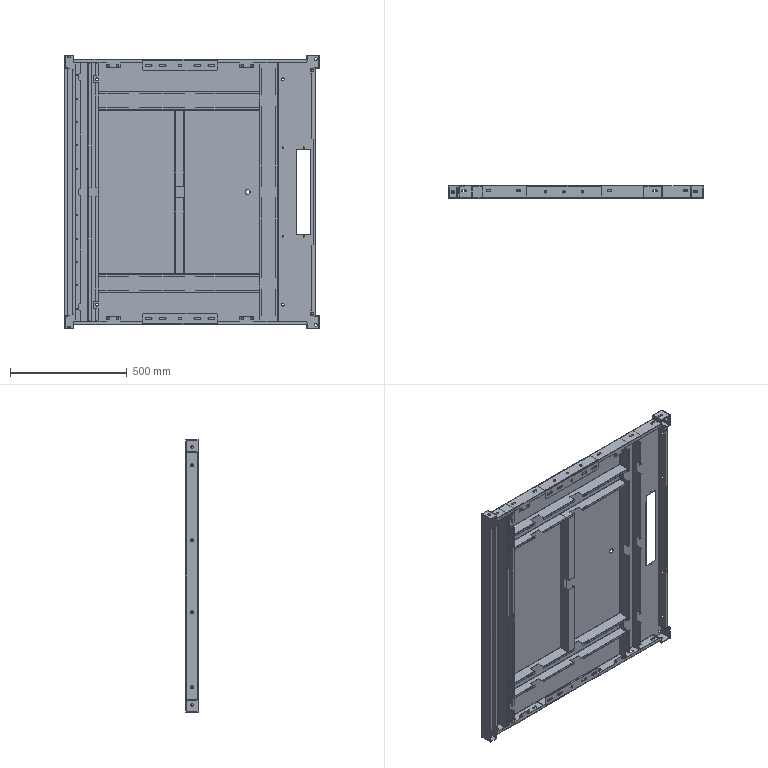Part | SolidWorks | features ReferencePattern 2, MirrorCompFeat 1 | 25 solids | 1396 faces | box 1093 x 53 x 1171 mm | volume 3806395 mm3 | plane 921 | cylinder 403 | cone 72 | commonest cylinder face diameters 10.5 x56 0.4 x55 9 x44 3.4 x41 10 x40 6 x30